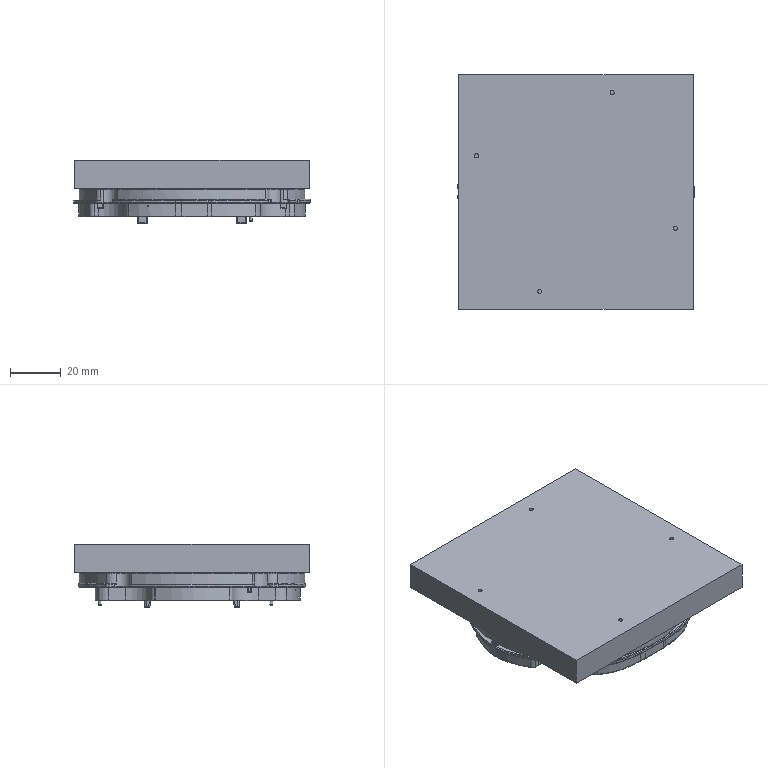NC program | NX | posted with a generic post | part box 92.935 x 92.1 x 24.829 mm
Lines 21645 to 23268 of 39008:
(PLANAR_MILL_7 , TOOL : D4-12-D4-50-3T-FINISH)
N43252 T12 M6
N43254 G54
N43256 G17 G0 G90 X-24.669 Y1.413 S4500 M3
N43258 G43 Z20. H12
N43260 Z-3.025
N43262 G94 G1 Z-6.025 F800.
N43264 X-25.476 Y-0.418
N43266 G2 X-24.68 Y-0.783 R27.9
N43268 G1 Y-0.533
N43270 G2 X-26.282 Y-0.078 R16.4
N43272 X-25.476 Y-0.418 R27.9
N43274 G1 X-26.443 Y-2.614
N43276 G2 X-24.23 Y-3.72 R25.5
N43278 X-22.28 Y-3.348 R12.08
N43280 G1 Y1.507
N43282 G2 X-25.753 Y2.28 R14.
N43284 G1 X-26.121 Y2.413
N43286 G2 X-26.538 Y2.571 R14.
N43288 X-28.778 Y1.718 R25.5
N43290 G3 X-28.876 Y1.255 R9.447
N43292 X-28.981 Y-0.229 R6.65
N43294 X-28.78 Y-1.719 R8.119
N43296 G2 X-26.443 Y-2.614 R25.5
N43298 G1 X-27.41 Y-4.811
N43300 G2 X-24.516 Y-6.338 R23.1
N43302 G1 X-24.286 Y-6.255
N43304 G2 X-20.999 Y-5.68 R9.68
N43306 G1 X-19.88
N43308 Y3.848
N43310 X-20.999
N43312 G2 X-24.938 Y4.537 R11.6
N43314 G1 X-25.306 Y4.67
N43316 G2 X-26.556 Y5.207 R11.6
N43318 X-30.71 Y3.646 R23.1
N43320 G3 X-30.928 Y2.962 R22.542
N43322 X-31.236 Y1.691 R11.847
N43324 X-31.379 Y-0.329 R9.05
N43326 X-31.059 Y-2.504 R10.519
N43328 X-30.726 Y-3.642 R17.948
N43330 G2 X-27.41 Y-4.811 R23.1
N43332 G1 X-28.378 Y-7.007
N43334 G2 X-24.764 Y-9.054 R20.7
N43336 X-23.839 Y-8.646 R7.28
N43338 G1 X-23.471 Y-8.513
N43340 G2 X-20.999 Y-8.08 R7.28
N43342 G1 X-17.999
N43344 G2 X-17.48 Y-8.098 R7.28
N43346 G1 Y6.263
N43348 G2 X-17.999 Y6.248 R9.2
N43350 G1 X-20.999
N43352 G2 X-24.123 Y6.795 R9.2
N43354 G1 X-24.491 Y6.928
N43356 G2 X-26.503 Y7.948 R9.2
N43358 X-32.518 Y5.681 R20.7
N43360 G3 X-33.226 Y3.654 R24.942
N43362 X-33.596 Y2.127 R14.247
N43364 X-33.777 Y-0.429 R11.45
N43366 X-33.383 Y-3.1 R12.919
N43368 X-32.536 Y-5.678 R20.348
N43370 G2 X-28.378 Y-7.007 R20.7
N43372 G1 X-29.345 Y-9.203
N43374 G2 X-24.823 Y-12.047 R18.3
N43376 X-23.024 Y-10.903 R4.88
N43378 G1 X-22.656 Y-10.77
N43380 G2 X-20.999 Y-10.48 R4.88
N43382 G1 X-17.999
N43384 G2 X-16.341 Y-10.77 R4.88
N43386 G1 X-15.973 Y-10.903
N43388 G2 X-15.08 Y-11.332 R4.88
N43390 G1 Y9.277
N43392 G2 X-15.321 Y9.185 R6.8
N43394 G1 X-15.689 Y9.052
N43396 G2 X-17.999 Y8.648 R6.8
N43398 G1 X-20.999
N43400 G2 X-23.308 Y9.052 R6.8
N43402 G1 X-23.676 Y9.185
N43404 G2 X-26.304 Y10.905 R6.8
N43406 X-34.231 Y7.82 R18.3
N43408 G3 X-34.85 Y6.309 R41.541
N43410 X-35.523 Y4.348 R27.342
N43412 X-35.956 Y2.563 R16.647
N43414 X-36.175 Y-0.528 R13.85
N43416 X-35.708 Y-3.696 R15.319
N43418 X-34.584 Y-7.003 R22.748
N43420 X-34.228 Y-7.821 R88.403
N43422 G2 X-29.345 Y-9.203 R18.3
N43424 G1 X-30.313 Y-11.4
N43426 G2 X-23.979 Y-16.442 R15.9
N43428 G1 Y-15.868
N43430 G2 X-23.839 Y-15.047 R2.48
N43432 G1 X-23.707 Y-14.672
N43434 G2 X-22.209 Y-13.16 R2.48
N43436 G1 X-21.841 Y-13.027
N43438 G2 X-20.999 Y-12.88 R2.48
N43440 G1 X-17.999
N43442 G2 X-17.156 Y-13.027 R2.48
N43444 G1 X-16.788 Y-13.16
N43446 G2 X-15.29 Y-14.672 R2.48
N43448 G1 X-15.158 Y-15.047
N43450 G2 X-15.019 Y-15.868 R2.48
N43452 G1 Y-18.001
N43454 G2 X-15.498 Y-19.621 R2.98
N43456 G1 X-7.442 Y-24.843
N43458 G2 X-8.76 Y-26.539 R12.58
N43460 G1 X-8.757 Y-26.548
N43462 G3 X-6.577 Y-26.732 R85.732
N43464 G1 X-5.951 Y-26.774
N43466 X-5.311 Y-26.812
N43468 G3 X-0.977 Y-26.958 R93.406
N43470 X3.366 Y-26.902 R93.502
N43472 X4.427 Y-26.858 R92.619
N43474 X5.477 Y-26.803 R92.484
N43476 X8.597 Y-26.572 R101.654
N43478 G1 X8.778 Y-26.555
N43480 G2 X7.445 Y-24.843 R12.58
N43482 G1 X-7.442
N43484 X-9.456 Y-23.538
N43486 G2 X-11.573 Y-25.897 R10.18
N43488 X-10.67 Y-28.754 R12.7
N43490 G3 X-10.159 Y-28.816 R22.91
N43492 X-6.742 Y-29.126 R88.132
N43494 G1 X-6.102 Y-29.169
N43496 X-5.451 Y-29.208
N43498 G3 X-1.002 Y-29.358 R95.806
N43500 X3.453 Y-29.3 R95.902
N43502 X4.539 Y-29.256 R95.019
N43504 X5.618 Y-29.199 R94.884
N43506 X8.812 Y-28.962 R104.054
N43508 X10.875 Y-28.718 R36.499
N43510 G2 X12.206 Y-26.37 R13.414
N43512 X8.842 Y-22.443 R10.18
N43514 G1 X-8.839
N43516 G2 X-9.456 Y-23.538 R10.18
N43518 G1 X-11.47 Y-22.232
N43520 G2 X-14.799 Y-25.092 R7.78
N43522 X-12.898 Y-30.092 R10.3
N43524 X-12.629 Y-30.858 R11.014
N43526 G3 X-10.423 Y-31.201 R25.31
N43528 X-6.907 Y-31.521 R90.532
N43530 G1 X-6.253 Y-31.564
N43532 X-5.591 Y-31.604
N43534 G3 X-1.028 Y-31.757 R98.206
N43536 X3.539 Y-31.699 R98.302
N43538 X4.652 Y-31.653 R97.419
N43540 X5.758 Y-31.595 R97.284
N43542 X9.026 Y-31.352 R106.454
N43544 X11.881 Y-30.989 R38.899
N43546 X12.634 Y-30.851 R20.991
N43548 G2 X16.026 Y-25.727 R11.014
N43550 G1 X16.029 Y-25.526
N43552 G2 X10.494 Y-20.043 R7.78
N43554 G1 X-10.491
N43556 G2 X-11.47 Y-22.232 R7.78
N43558 G1 X-13.484 Y-20.927
N43560 G2 X-17.999 Y-23.381 R5.38
N43562 G1 X-18.603
N43564 G2 X-18.46 Y-24.767 R18.3
N43566 X-15.26 Y-30.663 R7.9
N43568 X-14.628 Y-32.852 R8.614
N43570 G3 X-13.772 Y-33.068 R18.345
N43572 X-10.686 Y-33.587 R27.71
N43574 X-7.072 Y-33.915 R92.932
N43576 G1 X-6.404 Y-33.959
N43578 X-5.73 Y-34.
N43580 G3 X-1.053 Y-34.157 R100.606
N43582 X3.626 Y-34.097 R100.702
N43584 X4.765 Y-34.05 R99.819
N43586 X5.898 Y-33.991 R99.684
N43588 X9.24 Y-33.743 R108.854
N43590 X12.272 Y-33.357 R41.299
N43592 X14.632 Y-32.842 R23.391
N43594 G2 X18.424 Y-26.925 R8.614
N43596 G1 Y-25.951
N43598 G2 X18.606 Y-23.381 R18.3
N43600 G1 X18.001
N43602 G2 X12.621 Y-18.001 R5.38
N43604 G1 Y-17.643
N43606 X-12.2
N43608 G2 X-12.619 Y-17.613 R2.88
N43610 G1 Y-18.001
N43612 G2 X-13.484 Y-20.927 R5.38
N43614 G1 X-15.498 Y-19.621
N43616 G2 X-17.999 Y-20.981 R2.98
N43618 G1 X-20.999
N43620 G2 X-21.642 Y-20.91 R2.98
N43622 G1 X-21.538 Y-20.442
N43624 G2 X-23.499 Y-18.001 R2.5
N43626 G1 Y-15.868
N43628 G2 X-23.386 Y-15.206 R2.
N43630 G1 X-23.254 Y-14.831
N43632 G2 X-22.046 Y-13.612 R2.
N43634 G1 X-21.678 Y-13.479
N43636 G2 X-20.999 Y-13.36 R2.
N43638 G1 X-17.999
N43640 G2 X-17.319 Y-13.479 R2.
N43642 G1 X-16.951 Y-13.612
N43644 G2 X-15.743 Y-14.831 R2.
N43646 G1 X-15.611 Y-15.206
N43648 G2 X-15.499 Y-15.868 R2.
N43650 G1 Y-18.001
N43652 G2 X-17.999 Y-20.501 R2.5
N43654 G1 X-20.999
N43656 G2 X-21.538 Y-20.442 R2.5
N43658 G1 X-21.642 Y-20.91
N43660 G2 X-20.821 Y-25.951 R15.9
N43662 G1 Y-26.142
N43664 G2 X-17.647 Y-31.234 R5.5
N43666 X-16.952 Y-34.618 R6.214
N43668 G3 X-16.606 Y-34.744 R15.995
N43670 X-14.302 Y-35.409 R20.745
N43672 X-10.95 Y-35.972 R30.11
N43674 X-7.237 Y-36.309 R95.332
N43676 G1 X-6.555 Y-36.355
N43678 X-5.87 Y-36.395
N43680 G3 X-1.078 Y-36.557 R103.006
N43682 X3.712 Y-36.496 R103.102
N43684 X4.877 Y-36.448 R102.219
N43686 X6.039 Y-36.387 R102.084
N43688 X9.455 Y-36.133 R111.254
N43690 X12.663 Y-35.725 R43.699
N43692 X15.887 Y-34.978 R25.791
N43694 X16.955 Y-34.616 R16.039
N43696 G2 X20.824 Y-28.364 R6.214
N43698 G1 Y-25.951
N43700 G2 X21.644 Y-20.91 R15.9
N43702 X21.001 Y-20.981 R2.98
N43704 G1 X18.001
N43706 G2 X15.021 Y-18.001 R2.98
N43708 G1 Y-15.868
N43710 G2 X15.101 Y-15.243 R2.48
N43712 G1 X-12.2
N43714 G2 X-12.68 Y-14.763 R0.48
N43716 G1 Y21.237
N43718 G2 X-12.29 Y21.708 R0.48
N43720 G1 X-13.189 Y26.423
N43722 G2 X-12.2 Y26.517 R5.28
N43724 G1 X15.186
N43726 G2 X14.518 Y27.284 R11.014
N43728 G1 X-14.992
N43730 X-14.954 Y27.209
N43732 G2 X-13.189 Y26.423 R9.7
N43734 G1 X-12.74 Y24.066
N43736 G2 X-12.2 Y24.117 R2.88
N43738 G1 X17.3
N43740 G2 X18.547 Y23.833 R2.88
N43742 X18.424 Y25.95 R18.3
N43744 G1 Y26.923
N43746 G2 X15.936 Y29.418 R8.614
N43748 X15.514 Y29.684 R7.8
N43750 G1 X-18.421
N43752 Y28.077
N43754 G2 X-16.692 Y25.182 R8.8
N43756 X-13.545 Y23.784 R7.3
N43758 X-12.74 Y24.066 R2.88
N43760 G1 X-12.29 Y21.708
N43762 X-12.2 Y21.717
N43764 X17.3
N43766 G2 X17.78 Y21.237 R0.48
N43768 G1 Y20.971
N43770 G2 X18.001 Y20.979 R2.98
N43772 G1 X21.001
N43774 G2 X21.644 Y20.909 R2.98
N43776 G1 X21.541 Y20.441
N43778 G2 X23.501 Y17.999 R2.5
N43780 G1 Y15.956
N43782 G2 X23.389 Y15.294 R2.
N43784 G1 X23.257 Y14.919
N43786 G2 X22.049 Y13.7 R2.
N43788 G1 X21.681 Y13.567
N43790 G2 X21.001 Y13.448 R2.
N43792 G1 X18.001
N43794 G2 X17.3 Y13.575 R2.
N43796 G1 Y-13.487
N43798 X17.322 Y-13.479
N43800 G2 X18.001 Y-13.36 R2.
N43802 G1 X21.001
N43804 G2 X21.681 Y-13.479 R2.
N43806 G1 X22.049 Y-13.612
N43808 G2 X23.257 Y-14.831 R2.
N43810 G1 X23.389 Y-15.206
N43812 G2 X23.501 Y-15.868 R2.
N43814 G1 Y-18.001
N43816 G2 X21.001 Y-20.501 R2.5
N43818 G1 X18.001
N43820 G2 X15.501 Y-18.001 R2.5
N43822 G1 Y-15.868
N43824 G2 X15.614 Y-15.206 R2.
N43826 G1 X15.746 Y-14.831
N43828 X15.771 Y-14.763
N43830 X-12.2
N43832 Y21.237
N43834 X17.3
N43836 Y20.399
N43838 G2 X18.001 Y20.499 R2.5
N43840 G1 X21.001
N43842 G2 X21.541 Y20.441 R2.5
N43844 G1 X21.644 Y20.909
N43846 G2 X20.824 Y25.95 R15.9
N43848 G1 Y28.363
N43850 G2 X17.654 Y31.226 R6.214
N43852 X16.326 Y32.084 R5.4
N43854 G1 X-20.821
N43856 Y27.072
N43858 G2 X-18.61 Y22.899 R6.4
N43860 G1 X-17.999
N43862 G2 X-13.099 Y17.999 R4.9
N43864 G1 Y15.956
N43866 G2 X-13.347 Y14.499 R4.4
N43868 G1 X-13.478 Y14.124
N43870 G2 X-16.136 Y11.443 R4.4
N43872 G1 X-16.504 Y11.31
N43874 G2 X-17.999 Y11.048 R4.4
N43876 G1 X-20.999
N43878 G2 X-22.493 Y11.31 R4.4
N43880 G1 X-22.861 Y11.443
N43882 G2 X-25.519 Y14.124 R4.4
N43884 G1 X-25.66 Y14.528
N43886 G2 X-35.848 Y10.074 R15.9
N43888 G1 X-36.099 Y9.526
N43890 G3 X-37.088 Y7.174 R43.941
N43892 X-37.821 Y5.041 R29.742
N43894 X-38.316 Y2.999 R19.047
N43896 X-38.573 Y-0.628 R16.25
N43898 X-38.033 Y-4.292 R17.719
N43900 X-36.79 Y-7.947 R25.148
N43902 X-35.847 Y-10.075 R90.803
N43904 G2 X-30.313 Y-11.4 R15.9
N43906 G1 X-31.28 Y-13.596
N43908 G2 X-23.221 Y-25.951 R13.5
N43910 G1 Y-28.028
N43912 G2 X-20.121 Y-31.804 R3.1
N43914 X-19.805 Y-35.964 R3.814
N43916 G3 X-17.403 Y-37.008 R18.395
N43918 X-14.833 Y-37.749 R23.145
N43920 X-11.213 Y-38.358 R32.51
N43922 X-7.406 Y-38.703 R97.732
N43924 X-6.706 Y-38.75 R99.978
N43926 X-6.002 Y-38.792 R101.452
N43928 X-1.103 Y-38.957 R105.406
N43930 X3.8 Y-38.894 R105.502
N43932 X4.99 Y-38.845 R104.619
N43934 X6.179 Y-38.782 R104.484
N43936 X9.669 Y-38.524 R113.654
N43938 X13.053 Y-38.093 R46.099
N43940 X16.577 Y-37.277 R28.191
N43942 X19.807 Y-35.963 R18.439
N43944 G2 X23.224 Y-30.314 R3.814
N43946 G1 Y-25.951
N43948 G2 X31.777 Y-13.39 R13.5
N43950 G1 X27.38 Y-2.225
N43952 G2 X28.781 Y-1.72 R25.5
N43954 G3 X28.879 Y-1.256 R9.444
N43956 X28.984 Y0.228 R6.652
N43958 X28.783 Y1.718 R8.116
N43960 G2 X27.38 Y2.224 R25.5
N43962 G1 Y-2.225
N43964 X28.259 Y-4.458
N43966 G2 X30.713 Y-3.647 R23.1
N43968 G3 X30.931 Y-2.963 R22.54
N43970 X31.239 Y-1.692 R11.844
N43972 X31.382 Y0.328 R9.052
N43974 X31.062 Y2.503 R10.516
N43976 X30.729 Y3.641 R17.951
N43978 G2 X24.98 Y6.058 R23.1
N43980 G1 Y-6.059
N43982 G2 X28.259 Y-4.458 R23.1
N43984 G1 X29.139 Y-6.691
N43986 G2 X32.521 Y-5.682 R20.7
N43988 G3 X33.229 Y-3.655 R24.94
N43990 X33.599 Y-2.128 R14.244
N43992 X33.78 Y0.427 R11.452
N43994 X33.386 Y3.099 R12.916
N43996 X32.539 Y5.677 R20.351
N43998 G2 X24.694 Y9.104 R20.7
N44000 X23.842 Y8.734 R7.28
N44002 G1 X23.474 Y8.601
N44004 G2 X22.58 Y8.341 R7.28
N44006 G1 Y-8.253
N44008 G2 X23.474 Y-8.513 R7.28
N44010 G1 X23.842 Y-8.646
N44012 G2 X24.767 Y-9.054 R7.28
N44014 X29.139 Y-6.691 R20.7
N44016 G1 X30.018 Y-8.924
N44018 G2 X34.234 Y-7.821 R18.3
N44020 G3 X34.852 Y-6.31 R41.545
N44022 X35.526 Y-4.349 R27.34
N44024 X35.959 Y-2.564 R16.644
N44026 X36.178 Y0.527 R13.852
N44028 X35.711 Y3.695 R15.316
N44030 X34.587 Y7.001 R22.751
N44032 X34.231 Y7.82 R88.394
N44034 G2 X24.777 Y12.088 R18.3
N44036 X23.027 Y10.991 R4.88
N44038 G1 X22.659 Y10.858
N44040 G2 X21.001 Y10.568 R4.88
N44042 G1 X20.18
N44044 Y-10.48
N44046 X21.001
N44048 G2 X22.659 Y-10.77 R4.88
N44050 G1 X23.027 Y-10.903
N44052 G2 X24.826 Y-12.047 R4.88
N44054 X30.018 Y-8.924 R18.3
N44056 G1 X30.898 Y-11.157
N44058 G2 X35.851 Y-10.075 R15.9
N44060 G1 X36.102 Y-9.527
N44062 G3 X37.091 Y-7.175 R43.945
N44064 X37.824 Y-5.042 R29.74
N44066 X38.319 Y-3. R19.044
N44068 X38.576 Y0.627 R16.252
N44070 X38.036 Y4.291 R17.716
N44072 X36.793 Y7.946 R25.151
N44074 X35.85 Y10.074 R90.794
N44076 G2 X23.981 Y16.44 R15.9
N44078 G1 Y15.956
N44080 G2 X23.842 Y15.135 R2.48
N44082 G1 X23.71 Y14.76
N44084 G2 X22.212 Y13.248 R2.48
N44086 G1 X21.844 Y13.115
N44088 G2 X21.001 Y12.968 R2.48
N44090 G1 X18.001
N44092 G2 X17.78 Y12.978 R2.48
N44094 G1 Y-12.89
N44096 G2 X18.001 Y-12.88 R2.48
N44098 G1 X21.001
N44100 G2 X21.844 Y-13.027 R2.48
N44102 G1 X22.212 Y-13.16
N44104 G2 X23.71 Y-14.672 R2.48
N44106 G1 X23.842 Y-15.047
N44108 G2 X23.981 Y-15.868 R2.48
N44110 G1 Y-16.442
N44112 G2 X30.898 Y-11.157 R15.9
N44114 G1 X31.777 Y-13.39
N44116 G2 X36.724 Y-12.451 R13.5
N44118 G1 X37.385
N44120 G3 X38.287 Y-10.521 R103.509
N44122 X39.329 Y-8.041 R46.345
N44124 X40.122 Y-5.736 R32.14
N44126 X40.679 Y-3.436 R21.444
N44128 X40.974 Y0.726 R18.652
N44130 X40.361 Y4.887 R20.116
N44132 X38.999 Y8.891 R27.551
N44134 X37.386 Y12.45 R93.194
N44136 G1 X36.724
N44138 G2 X23.224 Y25.95 R13.5
N44140 G1 Y30.313
N44142 G2 X19.457 Y33.172 R3.814
N44144 X17.389 Y34.484 R3.
N44146 G1 X-21.326
N44148 G3 X-22.74 Y34.046 R2.5
N44150 X-23.221 Y32.944 R1.5
N44152 G1 Y26.097
N44154 G3 X-22.971 Y25.664 R0.5
N44156 G2 X-21.364 Y20.473 R4.
N44158 X-20.999 Y20.499 R2.5
N44160 G1 X-17.999
N44162 G2 X-15.499 Y17.999 R2.5
N44164 G1 Y15.956
N44166 G2 X-15.611 Y15.294 R2.
N44168 G1 X-15.743 Y14.919
N44170 G2 X-16.951 Y13.7 R2.
N44172 G1 X-17.319 Y13.567
N44174 G2 X-17.999 Y13.448 R2.
N44176 G1 X-20.999
N44178 G2 X-21.678 Y13.567 R2.
N44180 G1 X-22.046 Y13.7
N44182 G2 X-23.254 Y14.919 R2.
N44184 G1 X-23.386 Y15.294
N44186 G2 X-23.499 Y15.956 R2.
N44188 G1 Y17.999
N44190 G2 X-23.448 Y18.501 R2.5
N44192 X-25.349 Y18.218 R4.
N44194 G3 X-25.799 Y18.015 R0.5
N44196 G2 X-36.721 Y12.45 R13.5
N44198 G1 X-37.382
N44200 G3 X-38.284 Y10.52 R103.527
N44202 X-39.327 Y8.04 R46.341
N44204 X-40.119 Y5.735 R32.142
N44206 X-40.676 Y3.435 R21.447
N44208 X-40.971 Y-0.727 R18.65
N44210 X-40.358 Y-4.888 R20.119
N44212 X-38.996 Y-8.892 R27.548
N44214 X-37.383 Y-12.451 R93.203
N44216 G1 X-36.721
N44218 G2 X-31.28 Y-13.596 R13.5
N44220 G1 X-30.474 Y-11.766
N44222 Z-3.025
N44224 G0 Z20.
(PLANAR_MILL_7_COPY_2 , TOOL : D4-12-D4-50-3T-FINISH)
N44226 X0.103 Y-27.363
N44228 Z-3.525
N44230 G1 Z-6.525
N44232 X0.105 Y-29.363
N44234 G3 X3.453 Y-29.3 R95.902
N44236 X4.539 Y-29.256 R95.019
N44238 X5.618 Y-29.199 R94.884
N44240 X7.299 Y-29.088 R116.954
N44242 X8.868 Y-28.954 R65.735
N44244 X10.877 Y-28.711 R43.493
N44246 G2 X11.209 Y-28.014 R13.414
N44248 X9.478 Y-26.589 R12.1
N44250 G1 X-9.475
N44252 G2 X-10.892 Y-27.793 R12.1
N44254 X-10.67 Y-28.752 R12.7
N44256 G3 X-10.023 Y-28.831 R24.468
N44258 X-6.743 Y-29.126 R89.057
N44260 G1 X-6.102 Y-29.169
N44262 X-5.447 Y-29.208
N44264 G3 X-1.002 Y-29.358 R95.806
N44266 X0.105 Y-29.363 R95.902
N44268 G1 X0.108 Y-31.763
N44270 G3 X3.539 Y-31.699 R98.302
N44272 X4.652 Y-31.653 R97.419
N44274 X5.758 Y-31.595 R97.284
N44276 X7.474 Y-31.482 R119.354
N44278 X9.101 Y-31.343 R68.135
N44280 X12.393 Y-30.902 R45.893
N44282 G1 X12.632 Y-30.859
N44284 G2 X14.662 Y-27.108 R11.014
N44286 X10.532 Y-24.189 R9.7
N44288 G1 X-10.529
N44290 G2 X-13.82 Y-26.755 R9.7
N44292 X-12.898 Y-30.092 R10.3
N44294 X-12.629 Y-30.857 R11.014
N44296 G3 X-10.282 Y-31.217 R26.868
N44298 X-6.908 Y-31.521 R91.457
N44300 G1 X-6.253 Y-31.564
N44302 X-5.586 Y-31.604
N44304 G3 X-1.028 Y-31.757 R98.206
N44306 X0.108 Y-31.763 R98.302
N44308 G1 X0.111 Y-34.163
N44310 G3 X3.626 Y-34.097 R100.702
N44312 X4.765 Y-34.05 R99.819
N44314 X5.898 Y-33.991 R99.684
N44316 X7.649 Y-33.875 R121.754
N44318 X9.333 Y-33.732 R70.535
N44320 X12.797 Y-33.267 R48.293
N44322 X14.63 Y-32.855 R18.15
N44324 G2 X18.424 Y-26.925 R8.614
N44326 G1 Y-25.951
N44328 G2 X18.436 Y-25.301 R18.3
N44330 G1 X18.001
N44332 G2 X11.762 Y-21.789 R7.3
N44334 G1 X-11.759
N44336 G2 X-17.813 Y-25.298 R7.3
N44338 X-15.26 Y-30.663 R7.9
N44340 X-14.627 Y-32.854 R8.614
N44342 G3 X-13.536 Y-33.12 R20.526
N44344 X-10.541 Y-33.603 R29.268
N44346 X-7.073 Y-33.915 R93.857
N44348 G1 X-6.404 Y-33.959
N44350 X-5.726 Y-34.
N44352 G3 X-1.053 Y-34.157 R100.606
N44354 X0.111 Y-34.163 R100.702
N44356 G1 X0.114 Y-36.563
N44358 G3 X3.712 Y-36.496 R103.102
N44360 X4.877 Y-36.448 R102.219
N44362 X6.039 Y-36.387 R102.084
N44364 X7.824 Y-36.269 R124.154
N44366 X9.566 Y-36.12 R72.935
N44368 X13.202 Y-35.633 R50.693
N44370 X16.376 Y-34.825 R20.55
N44372 X16.955 Y-34.616 R17.313
N44374 G2 X20.824 Y-28.364 R6.214
N44376 G1 Y-25.951
N44378 G2 X21.12 Y-22.899 R15.9
N44380 G1 X18.001 Y-22.901
N44382 G2 X13.302 Y-19.389 R4.9
N44384 G1 X-13.299
N44386 G2 X-17.999 Y-22.901 R4.9
N44388 G1 X-21.117 Y-22.899
N44390 G2 X-20.821 Y-25.951 R15.9
N44392 G1 Y-26.142
N44394 G2 X-17.647 Y-31.234 R5.5
N44396 X-16.952 Y-34.618 R6.214
N44398 G3 X-16.378 Y-34.826 R17.312
N44400 X-15.24 Y-35.175 R18.745
N44402 X-14.041 Y-35.466 R22.926
N44404 X-10.8 Y-35.989 R31.668
N44406 X-7.238 Y-36.309 R96.257
N44408 G1 X-6.555 Y-36.355
N44410 X-5.865 Y-36.396
N44412 G3 X-1.078 Y-36.557 R103.006
N44414 X0.114 Y-36.563 R103.102
N44416 G1 X0.116 Y-38.963
N44418 G3 X3.8 Y-38.894 R105.502
N44420 X4.99 Y-38.845 R104.619
N44422 X6.179 Y-38.782 R104.484
N44424 X7.999 Y-38.662 R126.554
N44426 X9.798 Y-38.509 R75.335
N44428 X13.606 Y-37.999 R53.093
N44430 X17.152 Y-37.097 R22.95
N44432 X18.506 Y-36.578 R19.713
N44434 X19.807 Y-35.962 R18.287
N44436 G1 X19.795 Y-35.941
N44438 G2 X23.224 Y-30.314 R3.814
N44440 G1 Y-25.951
N44442 G2 X26.628 Y-16.989 R13.5
N44444 G1 X23.501
N44446 Y-18.001
N44448 G2 X21.001 Y-20.501 R2.5
N44450 G1 X18.001
N44452 G2 X15.501 Y-18.001 R2.5
N44454 G1 Y-16.989
N44456 X-15.499
N44458 Y-18.001
N44460 G2 X-17.999 Y-20.501 R2.5
N44462 G1 X-20.999
N44464 G2 X-23.499 Y-18.001 R2.5
N44466 G1 Y-16.989
N44468 X-26.625
N44470 G2 X-23.221 Y-25.951 R13.5
N44472 G1 Y-28.028
N44474 G2 X-20.121 Y-31.804 R3.1
N44476 X-19.805 Y-35.964 R3.814
N44478 G3 X-18.506 Y-36.579 R18.312
N44480 X-17.154 Y-37.097 R19.712
N44482 X-15.87 Y-37.49 R21.145
N44484 X-14.545 Y-37.813 R25.326
N44486 X-11.059 Y-38.375 R34.068
N44488 X-7.407 Y-38.703 R98.657
N44490 X-6.706 Y-38.75 R101.242
N44492 X-6.002 Y-38.792 R105.477
N44494 X-1.103 Y-38.957 R105.406
N44496 X0.116 Y-38.963 R105.502
N44498 G1 X0.114 Y-36.963
N44500 Z-3.525
N44502 G0 Z20.
(PLANAR_MILL_7_COPY , TOOL : D4-12-D4-50-3T-FINISH)
N44504 X1.8 Y7.097
N44506 Z-5.125
N44508 G1 Y-0.763 Z-5.813
N44510 X3.3 Z-5.944
N44512 Y7.237 Z-6.644
N44514 X1.8 Z-6.776
N44516 Y3.237 Z-7.125
N44518 Y-0.763
N44520 X3.3
N44522 Y7.237
N44524 X1.8
N44526 Y3.237
N44528 X-0.6
N44530 Y-3.163
N44532 X5.7
N44534 Y9.637
N44536 X-0.6
N44538 Y3.237
N44540 X-3.
N44542 Y-5.563
N44544 X8.1
N44546 Y12.037
N44548 X-3.
N44550 Y3.237
N44552 X-5.4
N44554 Y-7.963
N44556 X10.5
N44558 Y14.437
N44560 X-5.4
N44562 Y3.237
N44564 X-7.8
N44566 Y-10.363
N44568 X12.9
N44570 Y16.837
N44572 X-7.8
N44574 Y3.237
N44576 X-10.2
N44578 Y-12.763
N44580 X15.3
N44582 Y19.237
N44584 X-10.2
N44586 Y3.237
N44588 Z-5.125
N44590 G0 Z20.
(PLANAR_MILL_8 , TOOL : D4-12-D4-50-3T-FINISH)
N44592 X2.722 Y-46.43
N44594 Z-5.025
N44596 G1 Z-8.025
N44598 X2.674 Y-44.431
N44600 G2 X-1.16 Y-44.457 R110.96
N44602 X-6.314 Y-44.283 R110.965
N44604 X-7.052 Y-44.239 R108.655
N44606 X-7.793 Y-44.19 R106.796
N44608 X-12.102 Y-43.79 R97.842
N44610 X-16.511 Y-43.005 R36.323
N44612 X-21.497 Y-41.252 R26.415
N44614 X-26.037 Y-38.46 R23.641
N44616 X-28.721 Y-32.949 R7.
N44618 G1 Y-25.951
N44620 G3 X-36.721 Y-17.951 R8.
N44622 G1 X-38.324
N44624 G2 X-41.921 Y-15.701 R4.
N44626 G1 X-42.093 Y-15.347
N44628 G2 X-43.314 Y-12.745 R107.036
N44630 X-44.45 Y-10.043 R52.936
N44632 X-45.371 Y-7.379 R38.019
N44634 X-46.063 Y-4.58 R26.791
N44636 X-46.464 Y1.056 R24.133
N44638 X-45.59 Y6.612 R25.715
N44640 X-43.934 Y11.334 R34.882
N44642 X-41.911 Y15.713 R101.663
N44644 X-38.321 Y17.95 R4.
N44646 G1 X-36.721
N44648 G3 X-28.721 Y25.95 R8.
N44650 G1 Y32.944
N44652 G2 X-26.183 Y38.338 R7.
N44654 G1 X-26.103 Y38.401
N44656 G2 X-21.637 Y39.978 R8.
N44658 G1 X-21.559 Y39.98
N44660 X21.332 Y39.984
N44662 G2 X26.107 Y38.403 R8.
N44664 G1 X26.189 Y38.339
N44666 G2 X28.724 Y32.947 R7.
N44668 G1 Y25.95
N44670 G3 X36.724 Y17.95 R8.
N44672 G1 X38.327
N44674 G2 X41.924 Y15.7 R4.
N44676 G1 X42.095 Y15.346
N44678 G2 X43.551 Y12.221 R104.577
N44680 X44.864 Y8.936 R45.111
N44682 X45.986 Y4.954 R31.184
N44684 X46.492 Y0.735 R23.963
N44686 G1 X46.504 Y0.002
N44688 X46.491 Y-0.763
N44690 G2 X46.117 Y-4.284 R23.947
N44692 X45.283 Y-7.675 R28.662
N44694 X43.727 Y-11.824 R38.944
N44696 X41.914 Y-15.714 R105.253
N44698 X38.324 Y-17.951 R4.
N44700 G1 X36.724
N44702 G3 X28.724 Y-25.951 R8.
N44704 G1 Y-32.946
N44706 G2 X26.04 Y-38.457 R7.
N44708 X23.669 Y-40.095 R24.159
N44710 X21.116 Y-41.439 R23.832
N44712 X18.415 Y-42.471 R24.557
N44714 X15.659 Y-43.199 R29.764
N44716 X11.031 Y-43.918 R41.738
N44718 X6.5 Y-44.273 R115.493
N44720 G1 X6.313 Y-44.284
N44722 X6.125 Y-44.294
N44724 X6. Y-44.301
N44726 X5.875 Y-44.308
N44728 X5.749 Y-44.314
N44730 G2 X5.499 Y-44.327 R110.292
N44732 G1 X5.374 Y-44.333
N44734 G2 X5.123 Y-44.345 R110.244
N44736 X4.372 Y-44.377 R110.125
N44738 X4.122 Y-44.386 R110.403
N44740 X2.674 Y-44.431 R110.96
N44742 G1 X2.722 Y-46.43
N44744 Z-5.025
N44746 G0 Z20.
(PLANAR_MILL_8_COPY , TOOL : D4-12-D4-50-3T-FINISH)
N44748 X-35.918 Y-27.373
N44750 Z-5.025
N44752 G1 Z-8.025
N44754 Y-25.373
N44756 X-36.918
N44758 G2 X-39.193 Y-23.098 R2.275
N44760 G1 Y-22.098
N44762 G2 X-36.918 Y-19.823 R2.275
N44764 G1 X-34.918
N44766 G2 X-32.643 Y-22.098 R2.275
N44768 G1 Y-23.098
N44770 G2 X-34.918 Y-25.373 R2.275
N44772 G1 X-35.918
N44774 Y-27.373
N44776 Z-5.025
N44778 G0 Z20.
N44780 X35.921
N44782 Z-5.025
N44784 G1 Z-8.025
N44786 Y-25.373
N44788 X34.921
N44790 G2 X32.646 Y-23.098 R2.275
N44792 G1 Y-22.098
N44794 G2 X34.921 Y-19.823 R2.275
N44796 G1 X36.921
N44798 G2 X39.196 Y-22.098 R2.275
N44800 G1 Y-23.098
N44802 G2 X36.921 Y-25.373 R2.275
N44804 G1 X35.921
N44806 Y-27.373
N44808 Z-5.025
N44810 G0 Z20.
(FLOOR_FACING_1 , TOOL : D4-12-D4-50-3T-FINISH)
N44812 X-44.494 Y-20.992
N44814 Z-5.025
N44816 G1 Z-8.025
N44818 X-40.117 Y-18.592
N44820 G2 X-38.76 Y-18.988 R1.
N44822 G1 X-38.115 Y-20.164
N44824 G2 X-36.918 Y-19.823 R2.275
N44826 G1 X-34.918
N44828 G2 X-32.643 Y-22.098 R2.275
N44830 G1 Y-22.907
N44832 G2 X-28.724 Y-25.755 R5.1
N44834 G3 X-36.721 Y-17.951 R8.
N44836 G1 X-38.324
N44838 G2 X-39.392 Y-17.806 R4.
N44840 G1 X-38.901 Y-18.731
N44842 X-38.76 Y-18.988
N44844 X-38.279 Y-19.865
N44846 G2 X-37.9 Y-19.812 R0.5
N44848 G1 X-43.475 Y-22.869
N44850 Z-5.025
N44852 G0 Z20.
N44854 X-12.095 Y48.505
N44856 Z-5.025
N44858 G1 Z-8.025
N44860 X-11.515 Y43.539
N44862 G2 X-12.392 Y42.43 R1.
N44864 G3 X-21.139 Y39.98 R27.062
N44866 G1 X21.106 Y39.984
N44868 X19.973 Y40.518
N44870 X18.048 Y41.221
N44872 X16.06 Y41.768
N44874 X14.018 Y42.185
N44876 X11.935 Y42.495
N44878 X9.825 Y42.722
N44880 X7.7 Y42.892
N44882 X3.303 Y43.107
N44884 Y41.583
N44886 X-3.297
N44888 Y43.111
N44890 X-6.417 Y42.974
N44892 X-9.758 Y42.737
N44894 X-12.392 Y42.43
N44896 X-13.067 Y42.351
N44898 X-13.383 Y42.295
N44900 G2 X-14.544 Y43.102 R1.
N44902 G1 X-15.427 Y48.023
N44904 Z-5.025
N44906 G0 Z20.
N44908 X34.277 Y36.865
N44910 Z-5.025
N44912 G1 Z-8.025
N44914 X30.54 Y33.549
N44916 G2 X29.129 Y33.633 R1.
N44918 G1 X28.608 Y34.22
N44920 G2 X28.724 Y32.947 R7.
N44922 G1 Y30.163
N44924 G2 X29.606 Y31.452 R5.1
N44926 G3 X29.65 Y33.046 R1.2
N44928 G1 X29.129 Y33.633
N44930 X28.608 Y34.22
N44932 G2 X28.644 Y34.008 R7.
N44934 G1 Z-5.025
N44936 G0 Z20.
N44938 X42.761 Y24.144
N44940 Z-5.025
N44942 G1 Z-8.025
N44944 X35.869 Y20.188
N44946 G3 X35.82 Y20.568 R0.5
N44948 G1 X35.581 Y20.983
N44950 X35.359 Y21.367
N44952 G2 X32.894 Y21.074 R6.9
N44954 G3 X36.276 Y19.766 R6.2
N44956 G1 X36.046 Y20.174
N44958 X35.82 Y20.568
N44960 X37.381 Y21.464
N44962 X37.14 Y21.883
N44964 X36.667 Y22.7
N44966 G3 X35.19 Y23.214 R1.2
N44968 G2 X28.727 Y25.753 R5.1
N44970 G3 X36.724 Y17.95 R8.
N44972 G1 X38.327
N44974 G2 X39.395 Y17.804 R4.
N44976 G1 X37.381 Y21.464
N44978 X37.14 Y21.883
N44980 X36.881 Y22.33
N44982 G2 X37.245 Y23.697 R1.
N44984 G1 X41.55 Y26.193
N44986 Z-5.025
N44988 G0 Z20.
N44990 X43.559 Y-22.72
N44992 Z-5.025
N44994 G1 Z-8.025
N44996 X39.165 Y-20.343
N44998 G2 X38.761 Y-18.988 R1.
N45000 G1 X39.392 Y-17.806
N45002 G2 X38.324 Y-17.951 R4.
N45004 G1 X36.724
N45006 G3 X28.727 Y-25.755 R8.
N45008 G2 X32.646 Y-22.907 R5.1
N45010 G1 Y-22.098
N45012 G2 X34.921 Y-19.823 R2.275
N45014 G1 X36.921
N45016 G2 X38.116 Y-20.162 R2.275
N45018 G1 X38.761 Y-18.988
N45020 X38.92 Y-18.693
N45022 X39.233 Y-18.106
N45024 G2 X39.909 Y-17.898 R0.5
N45026 G1 X44.769 Y-20.467
N45028 Z-5.025
N45030 G0 Z20.
N45032 X32.999 Y-38.314
N45034 Z-5.025
N45036 G1 Z-8.025
N45038 X29.231 Y-35.032
N45040 G2 X29.134 Y-33.621 R1.
N45042 G1 X29.661 Y-33.016
N45044 G3 X29.6 Y-31.446 R1.2
N45046 G2 X28.724 Y-30.164 R5.1
N45048 G1 Y-32.946
N45050 G2 X28.606 Y-34.227 R7.
N45052 G1 X29.134 Y-33.621
N45054 X29.661 Y-33.016
N45056 X29.771 Y-32.853
N45058 G2 X31.132 Y-32.469 R1.
N45060 G1 X35.433 Y-34.879
N45062 Z-5.025
N45064 G0 Z20.
N45066 X-34.224 Y-36.914
N45068 Z-5.025
N45070 G1 Z-8.025
N45072 X-30.553 Y-33.573
N45074 G2 X-29.14 Y-33.64 R1.
N45076 G1 X-28.603 Y-34.232
N45078 G2 X-28.721 Y-32.949 R7.
N45080 G1 Y-30.164
N45082 G2 X-29.599 Y-31.448 R5.1
N45084 G3 X-29.653 Y-33.026 R1.2
N45086 G1 X-29.387 Y-33.348
N45088 X-29.14 Y-33.64
N45090 X-28.603 Y-34.232
N45092 G2 X-28.637 Y-34.034 R7.
N45094 G1 Z-5.025
N45096 G0 Z20.
N45098 X-42.391 Y24.778
N45100 Z-5.025
N45102 G1 Z-8.025
N45104 X-35.512 Y20.802
N45106 G3 X-35.814 Y20.568 R0.5
N45108 G1 X-36.116 Y20.041
N45110 X-36.271 Y19.766
N45112 G3 X-32.892 Y21.074 R6.2
N45114 G2 X-35.353 Y21.366 R6.9
N45116 G1 X-35.446 Y21.207
N45118 X-35.814 Y20.568
N45120 X-37.377 Y21.462
N45122 X-39.388 Y17.805
N45124 G2 X-38.321 Y17.95 R4.
N45126 G1 X-36.721
N45128 G3 X-28.724 Y25.753 R8.
N45130 G2 X-35.184 Y23.213 R5.1
N45132 G3 X-36.659 Y22.7 R1.2
N45134 G1 X-37.003 Y22.109
N45136 X-37.377 Y21.462
N45138 X-37.681 Y20.93
N45140 X-37.871 Y20.593
N45142 G2 X-39.234 Y20.213 R1.
N45144 G1 X-43.584 Y22.669
N45146 Z-5.025
N45148 G0 Z20.
N45150 X-33.03 Y38.296
N45152 Z-5.025
N45154 G1 Z-8.025
N45156 X-29.236 Y35.044
N45158 G2 X-29.127 Y33.634 R1.
N45160 G1 X-29.656 Y33.017
N45162 G3 X-29.597 Y31.445 R1.2
N45164 G2 X-28.721 Y30.163 R5.1
N45166 G1 Y32.944
N45168 G2 X-28.598 Y34.251 R7.
N45170 G1 X-29.127 Y33.634
N45172 X-29.656 Y33.017
N45174 X-29.762 Y32.863
N45176 G2 X-31.127 Y32.494 R1.
N45178 G1 X-35.402 Y34.949
N45180 Z-5.025
N45182 G0 Z20.
(PLANAR_MILL_10 , TOOL : D4-12-D4-50-3T-FINISH)
N45184 X-18.729 Y32.784
N45186 Z0.375
N45188 G1 Z-2.625
N45190 Y36.784
N45192 X-20.729
N45194 X-21.326
N45196 G3 X-24.167 Y35.853 R4.8
N45198 X-25.521 Y32.944 R3.8
N45200 G1 Y26.097
N45202 G3 X-24.121 Y23.672 R2.8
N45204 G2 X-25.132 Y20.507 R1.7
N45206 G3 X-27.659 Y19.369 R2.8
N45208 G2 X-36.721 Y14.75 R11.2
N45210 G1 X-38.009
N45212 G3 X-39.177 Y14.019 R1.3
N45214 X-41.384 Y9.107 R85.691
N45216 X-42.913 Y3.969 R26.452
N45218 X-43.284 Y-0.191 R21.168
N45220 X-42.84 Y-4.345 R21.641
N45222 X-41.331 Y-9.25 R26.958
N45224 X-39.18 Y-14.02 R88.056
N45226 X-38.011 Y-14.751 R1.3
N45228 G1 X-36.721
N45230 G2 X-25.521 Y-25.951 R11.2
N45232 G1 Y-28.591
N45234 G3 X-25.231 Y-29.572 R1.8
N45236 G1 Z0.375
N45238 G0 Z20.
N45240 X-18.354 Y-31.4
N45242 Z0.375
N45244 G1 Z-2.625
N45246 X-21.835 Y-33.371
N45248 G2 X-21.82 Y-34.856 R1.514
N45250 G3 X-20.869 Y-38.003 R2.3
N45252 X-18.998 Y-38.862 R20.233
N45254 X-17.054 Y-39.54 R23.615
N45256 X-12.359 Y-40.53 R28.493
N45258 X-6.133 Y-41.088 R91.573
N45260 X-3.295 Y-41.212 R107.536
N45262 X-2.908 Y-41.224 R107.659
N45264 X1.456 Y-41.253 R107.441
N45266 X3.882 Y-41.193 R107.66
N45268 X4.464 Y-41.17 R107.763
N45270 X6.313 Y-41.078 R105.797
N45272 X8.558 Y-40.928 R137.244
N45274 X10.798 Y-40.722 R67.482
N45276 X15.976 Y-39.829 R42.061
N45278 X20.871 Y-38.001 R21.135
N45280 X21.823 Y-34.855 R2.3
N45282 G2 X23.179 Y-32.613 R1.514
N45284 G3 X25.524 Y-30.314 R2.3
N45286 G1 Y-25.951
N45288 G2 X36.724 Y-14.751 R11.2
N45290 G1 X38.012
N45292 G3 X39.18 Y-14.021 R1.3
N45294 X41.414 Y-9.038 R84.756
N45296 X42.943 Y-3.824 R26.205
N45298 X43.287 Y0.263 R21.075
N45300 X42.843 Y4.343 R21.659
N45302 X41.334 Y9.248 R26.963
N45304 X39.183 Y14.018 R88.065
N45306 X38.014 Y14.75 R1.3
N45308 G1 X36.724
N45310 G2 X25.524 Y25.95 R11.2
N45312 G1 Y30.313
N45314 G3 X23.179 Y32.612 R2.3
N45316 G2 X21.652 Y33.904 R1.514
N45318 G1 X21.637 Y33.993
N45320 X18.164 Y31.769
N45322 Z0.375
N45324 G0 Z20.
N45326 X16.601 Y32.784
N45328 Z0.375
N45330 G1 Z-2.625
N45332 X17.634 Y36.784
N45334 X-13.201
N45336 X-15.201
N45338 Y32.784
N45340 Z0.375
N45342 G0 Z20.
(FLOOR_FACING_1_COPY , TOOL : D4-12-D4-50-3T-FINISH)
N45344 X-27.79 Y-40.516
N45346 Z0.375
N45348 G1 Z-2.625
N45350 X-24.933 Y-36.43
N45352 G2 X-23.54 Y-36.184 R1.
N45354 G1 X-23.057 Y-36.521
N45356 G2 X-22.696 Y-34.374 R3.3
N45358 G3 X-22.752 Y-33.798 R0.514
N45360 G1 X-22.828 Y-33.707
N45362 G2 X-25.421 Y-32.385 R2.6
N45364 G1 Y-32.949
N45366 G3 X-24.022 Y-35.846 R3.7
N45368 G1 X-23.54 Y-36.184
N45370 X-23.057 Y-36.521
N45372 G2 X-23.101 Y-36.112 R3.3
N45374 X-22.147 Y-35.069 R1.
N45376 G1 X-16.67 Y-34.822
N45378 Z0.375
N45380 G0 Z20.
N45382 X30.251 Y29.208
N45384 Z0.375
N45386 G1 Z-2.625
N45388 X22.962 Y33.13
N45390 G2 X22.555 Y34.485 R1.
N45392 G1 X22.645 Y34.026
N45394 G3 X23.159 Y33.612 R0.514
N45396 G2 X25.424 Y32.772 R3.3
N45398 G1 Y32.947
N45400 G3 X24.11 Y35.776 R3.7
N45402 X22.726 Y36.473 R4.7
N45404 G2 X22.465 Y34.943 R2.6
N45406 G1 X22.555 Y34.485
N45408 X22.645 Y34.026
N45410 G3 X22.978 Y33.641 R0.514
N45412 G2 X23.588 Y32.365 R1.
N45414 G1 X21.95 Y27.723
N45416 Z0.375
N45418 G0 Z20.
N45420 X-31.426 Y25.309
N45422 Z0.375
N45424 G1 Z-2.625
N45426 X-26.605 Y23.771
N45428 G2 X-25.956 Y22.514 R1.
N45430 X-26.383 Y21.389 R11.3
N45432 X-25.038 Y21.503 R3.8
N45434 G3 X-24.621 Y22.806 R0.7
N45436 G2 X-25.652 Y23.678 R3.8
N45438 X-25.956 Y22.514 R11.3
N45440 X-26.302 Y21.576 R11.3
N45442 X-27.611 Y21.041 R1.
N45444 G1 X-32.174 Y22.957
N45446 Z0.375
N45448 G0 Z20.
N45450 X26.133 Y-41.666
N45452 Z0.375
N45454 G1 Z-2.625
N45456 X23.292 Y-37.568
N45458 G2 X23.544 Y-36.177 R1.
N45460 G1 X24.027 Y-35.842
N45462 G3 X25.424 Y-32.946 R3.7
N45464 G1 Y-32.773
N45466 G2 X23.159 Y-33.613 R3.3
N45468 G3 X22.699 Y-34.374 R0.514
N45470 G2 X23.061 Y-36.512 R3.3
N45472 G1 X23.544 Y-36.177
N45474 X24.027 Y-35.842
N45476 G3 X24.335 Y-35.568 R3.7
N45478 G2 X25.749 Y-35.571 R1.
N45480 G1 X29.24 Y-39.078
N45482 Z0.375
N45484 G0 Z20.
(FLOOR_FACING_1_COPY_COPY , TOOL : D4-12-D4-50-3T-FINISH)
N45486 X31.946 Y-22.073
N45488 Z-4.025
N45490 G1 Z-6.025
N45492 G3 X32.946 Y-23.073 R1.
N45494 G1 X38.896
N45496 G3 X39.896 Y-22.073 R1.
N45498 G1 Z-4.025
N45500 G0 Z20.
N45502 X14.801 Y-16.866
N45504 Z2.
N45506 G1 Z0.
N45508 G3 X15.801 Y-17.866 R1.
N45510 G1 X23.201
N45512 G3 X24.201 Y-16.866 R1.
N45514 G1 Z2.
N45516 G0 Z20.
N45518 X14.801 Y18.199
N45520 Z2.
N45522 G1 Z0.
N45524 G3 X15.801 Y17.199 R1.
N45526 G1 X23.201
N45528 G3 X24.201 Y18.199 R1.
N45530 G1 Z2.
N45532 G0 Z20.
N45534 X16.7 Y36.718
N45536 Z0.975
N45538 G1 Z-1.025
N45540 Y36.625
N45542 G3 X17.7 Y35.625 R1.
N45544 G1 X22.599 Y35.626
N45546 G3 X23.599 Y36.626 R1.
N45548 G1 Y36.718
N45550 Z0.975
N45552 G0 Z20.
N45554 X-24.199 Y18.199
N45556 Z2.
N45558 G1 Z0.
N45560 G3 X-23.199 Y17.199 R1.
N45562 G1 X-15.799
N45564 G3 X-14.799 Y18.199 R1.
N45566 G1 Z2.
N45568 G0 Z20.
N45570 X-24.199 Y-16.866
N45572 Z2.
N45574 G1 Z0.
N45576 G3 X-23.199 Y-17.866 R1.
N45578 G1 X-15.799
N45580 G3 X-14.799 Y-16.866 R1.
N45582 G1 Z2.
N45584 G0 Z20.
N45586 X-26.596 Y-30.534
N45588 Z0.975
N45590 G1 Z-1.025
N45592 Y-30.627
N45594 G3 X-25.596 Y-31.627 R1.
N45596 G1 X-20.697
N45598 G3 X-19.697 Y-30.626 R1.
N45600 G1 Y-30.534
N45602 Z0.975
N45604 G0 Z20.
N45606 X-39.893 Y-22.073
N45608 Z-4.025
N45610 G1 Z-6.025
N45612 G3 X-38.893 Y-23.073 R1.
N45614 G1 X-32.943
N45616 G3 X-31.943 Y-22.073 R1.
N45618 G1 Z-4.025
N45620 G0 Z20.
(PLANAR_MILL_10_COPY , TOOL : D4-12-D4-50-3T-FINISH)
N45622 X15.549 Y34.125
N45624 Z-0.625
N45626 G1 Z-2.625
N45628 G3 X17.549 Y36.125 R2.
N45630 G2 X20.149 Y38.725 R2.6
N45632 X17.549 Y36.125 R-2.6
N45634 G3 X15.549 Y38.125 R2.
N45636 G1 Z-0.625
N45638 G0 Z20.
N45640 X-18.546 Y-29.127
N45642 Z-0.625
N45644 G1 Z-2.625
N45646 G3 X-20.546 Y-31.127 R2.
N45648 G2 X-23.146 Y-33.727 R2.6
N45650 X-20.546 Y-31.127 R-2.6
N45652 G3 X-18.546 Y-33.127 R2.
N45654 G1 Z-0.625
N45656 G0 Z20.
(PLANAR_MILL_11 , TOOL : D4-12-D4-50-3T-FINISH)
N45658 X-22.675 Y40.939
N45660 Z-2.125
N45662 G1 Z-4.125
N45664 G3 X-21.637 Y39.978 R1.
N45666 G2 X-18.612 Y37.719 R3.
N45668 G1 X-18.564 Y37.562
N45670 G2 X-18.429 Y36.784 R2.3
N45672 G1 X-15.501
N45674 G2 X-15.366 Y37.562 R2.3
N45676 G1 X-15.317 Y37.72
N45678 G2 X-12.409 Y39.984 R3.
N45680 G3 X-11.409 Y40.984 R1.
N45682 G1 Z-2.125
N45684 G0 Z20.
(PLANAR_MILL_11_COPY , TOOL : D4-12-D4-50-3T-FINISH)
N45686 X-22.675 Y40.939
N45688 Z-2.125
N45690 G1 Z-4.125
N45692 G3 X-21.637 Y39.978 R1.
N45694 G2 X-18.612 Y37.719 R3.
N45696 G1 X-18.564 Y37.562
N45698 G2 X-20.729 Y34.484 R2.3
N45700 G3 X-21.729 Y33.484 R1.
N45702 G1 Z-2.125
N45704 G0 Z20.
N45706 X-12.201
N45708 Z-2.125
N45710 G1 Z-4.125
N45712 G3 X-13.201 Y34.484 R1.
N45714 G2 X-15.366 Y37.562 R2.3
N45716 G1 X-15.317 Y37.72
N45718 G2 X-12.409 Y39.984 R3.
N45720 G3 X-11.409 Y40.984 R1.
N45722 G1 Z-2.125
N45724 G0 Z20.
N45726 M5
(PLANAR_MILL_7_COPY_1 , TOOL : D3-9-D4-50-3T-ROUGH)
N45728 T15 M6
N45730 G54
N45732 G17 G0 G90 X0.001 Y-37.963 S4500 M3
N45734 G43 Z20. H15
N45736 Z-3.025
N45738 G94 G1 Z-6.025 F600.
N45740 Y-39.463
N45742 G3 X3.818 Y-39.394 R106.002
N45744 X5.013 Y-39.345 R105.119
N45746 X6.208 Y-39.282 R104.984
N45748 X9.714 Y-39.022 R114.154
N45750 X13.134 Y-38.587 R46.599
N45752 X16.721 Y-37.756 R28.691
N45754 X20.038 Y-36.406 R18.939
N45756 X20.245 Y-35.722 R0.5
N45758 G2 X23.215 Y-30.814 R3.314
N45760 G3 X23.724 Y-30.314 R0.5
N45762 G1 Y-25.951
N45764 G2 X36.724 Y-12.951 R13.
N45766 G1 X37.699
N45768 G3 X38.742 Y-10.728 R104.009
N45770 X39.796 Y-8.221 R46.845
N45772 X40.6 Y-5.88 R32.64
N45774 X41.171 Y-3.527 R21.944
N45776 X41.473 Y0.747 R19.152
N45778 X40.845 Y5.011 R20.616
N45780 X39.459 Y9.088 R28.051
N45782 X37.701 Y12.95 R93.694
N45784 G1 X36.724
N45786 G2 X23.724 Y25.95 R13.
N45788 G1 Y30.313
N45790 G3 X23.215 Y30.813 R0.5
N45792 G2 X19.871 Y33.641 R3.314
N45794 X17.674 Y34.984 R2.5
N45796 G1 X-21.326
N45798 G3 X-23.051 Y34.438 R3.
N45800 X-23.721 Y32.944 R2.
N45802 G1 Y26.097
N45804 G3 X-23.221 Y25.231 R1.
N45806 G2 X-25.302 Y18.715 R3.5
N45808 G3 X-26.203 Y18.31 R1.
N45810 G2 X-36.721 Y12.95 R13.
N45812 G1 X-37.696
N45814 G3 X-38.739 Y10.727 R104.027
N45816 X-39.793 Y8.22 R46.841
N45818 X-40.597 Y5.879 R32.642
N45820 X-41.168 Y3.526 R21.947
N45822 X-41.47 Y-0.748 R19.15
N45824 X-40.842 Y-5.012 R20.619
N45826 X-39.456 Y-9.089 R28.048
N45828 X-37.698 Y-12.951 R93.703
N45830 G1 X-36.721
N45832 G2 X-23.721 Y-25.951 R13.
N45834 G1 Y-28.591
N45836 G2 X-20.671 Y-31.923 R2.6
N45838 X-20.243 Y-35.723 R3.314
N45840 G3 X-20.036 Y-36.408 R0.5
N45842 X-17.569 Y-37.479 R18.895
N45844 X-14.944 Y-38.237 R23.645
N45846 X-11.268 Y-38.855 R33.01
N45848 X-7.442 Y-39.202 R98.232
N45850 X-6.737 Y-39.249 R100.478
N45852 X-6.031 Y-39.291 R101.952
N45854 X-1.108 Y-39.457 R105.906
N45856 X0.001 Y-39.463 R106.002
N45858 G1 Y-37.963
N45860 Z-3.025
N45862 G0 Z20.
N45864 M5
(PLANAR_MILL_9 , TOOL : D3-9-D4-50-3T-ROUGH)
N45866 T17 M6
N45868 G54
N45870 G17 G0 G90 X2.618 Y-45.132 S4500 M3
N45872 G43 Z20. H17
N45874 Z0.075
N45876 G94 G1 Z-2.925 F600.
N45878 G41 X2.583 Y-43.632 D17
N45880 G2 X-1.152 Y-43.657 R110.16
N45882 X-6.268 Y-43.484 R110.167
N45884 X-7.002 Y-43.441 R106.979
N45886 X-7.736 Y-43.392 R107.145
N45888 X-12.01 Y-42.996 R97.042
N45890 X-16.322 Y-42.228 R35.523
N45892 X-21.157 Y-40.527 R25.615
N45894 X-25.544 Y-37.83 R22.841
N45896 X-27.921 Y-32.949 R6.2
N45898 G1 Y-25.951
N45900 G3 X-36.721 Y-17.151 R8.8
N45902 G1 X-38.324
N45904 G2 X-41.201 Y-15.351 R3.2
N45906 G1 X-41.373 Y-14.998
N45908 G2 X-42.586 Y-12.415 R106.236
N45910 X-43.704 Y-9.754 R52.136
N45912 X-44.606 Y-7.146 R37.219
N45914 X-45.277 Y-4.43 R25.991
N45916 X-45.665 Y1.019 R23.333
N45918 X-44.818 Y6.402 R24.915
N45920 X-43.2 Y11.016 R34.082
N45922 X-41.193 Y15.36 R100.863
N45924 X-38.321 Y17.15 R3.2
N45926 G1 X-36.721
N45928 G3 X-27.921 Y25.95 R8.8
N45930 G1 Y32.944
N45932 G2 X-25.681 Y37.715 R6.2
N45934 G1 X-25.617 Y37.765
N45936 G2 X-21.605 Y39.179 R7.2
N45938 X-19.388 Y37.522 R2.2
N45940 G3 X-19.317 Y37.292 R2.5
N45942 G2 X-20.729 Y35.284 R1.5
N45944 G1 X-21.326
N45946 G3 X-23.238 Y34.674 R3.3
N45948 X-24.021 Y32.944 R2.3
N45950 G1 Y26.097
N45952 G3 X-23.371 Y24.971 R1.3
N45954 G2 X-25.273 Y19.014 R3.2
N45956 G3 X-26.446 Y18.487 R1.3
N45958 G2 X-36.721 Y13.25 R12.7
N45960 G1 X-37.884
N45962 G3 X-39.012 Y10.851 R104.327
N45964 X-40.073 Y8.328 R47.141
N45966 X-40.885 Y5.966 R32.942
N45968 X-41.463 Y3.58 R22.247
N45970 X-41.77 Y-0.76 R19.45
N45972 X-41.133 Y-5.087 R20.919
N45974 X-39.732 Y-9.207 R28.348
N45976 X-37.886 Y-13.251 R94.003
N45978 G1 X-36.721
N45980 G2 X-24.021 Y-25.951 R12.7
N45982 G1 Y-28.591
N45984 G3 X-23.655 Y-28.884 R0.3
N45986 G2 X-20.957 Y-31.831 R2.3
N45988 G3 X-20.895 Y-32.123 R0.3
N45990 G2 X-20.506 Y-35.579 R3.014
N45992 G3 X-20.175 Y-36.673 R0.8
N45994 X-17.669 Y-37.762 R19.195
N45996 X-15.01 Y-38.529 R23.945
N45998 X-11.301 Y-39.153 R33.31
N46000 X-7.463 Y-39.501 R98.532
N46002 X-6.756 Y-39.548 R100.778
N46004 X-6.048 Y-39.591 R102.252
N46006 X-1.111 Y-39.757 R106.206
N46008 X3.828 Y-39.694 R106.302
N46010 X5.027 Y-39.644 R105.419
N46012 X6.226 Y-39.581 R105.284
N46014 X9.74 Y-39.32 R114.454
N46016 X13.183 Y-38.883 R46.899
N46018 X16.807 Y-38.043 R28.991
N46020 X20.177 Y-36.672 R19.239
N46022 X20.508 Y-35.577 R0.8
N46024 G2 X23.209 Y-31.114 R3.014
N46026 G3 X24.024 Y-30.314 R0.8
N46028 G1 Y-25.951
N46030 G2 X36.724 Y-13.251 R12.7
N46032 G1 X37.887
N46034 G3 X39.015 Y-10.852 R104.309
N46036 X40.076 Y-8.329 R47.145
N46038 X40.888 Y-5.967 R32.94
N46040 X41.466 Y-3.581 R22.244
N46042 X41.773 Y0.759 R19.452
N46044 X41.136 Y5.085 R20.916
N46046 X39.735 Y9.206 R28.351
N46048 X37.889 Y13.25 R93.994
N46050 G1 X36.724
N46052 G2 X24.024 Y25.95 R12.7
N46054 G1 Y30.313
N46056 G3 X23.209 Y31.112 R0.8
N46058 G2 X20.168 Y33.685 R3.014
N46060 G3 X19.874 Y33.941 R0.3
N46062 G2 X17.864 Y35.284 R2.2
N46064 G1 X-13.201
N46066 G2 X-14.613 Y37.292 R1.5
N46068 G3 X-14.542 Y37.524 R2.5
N46070 G2 X-12.409 Y39.184 R2.2
N46072 G1 X21.332
N46074 G2 X25.621 Y37.767 R7.2
N46076 G1 X25.686 Y37.716
N46078 G2 X27.924 Y32.947 R6.2
N46080 G1 Y25.95
N46082 G3 X36.724 Y17.15 R8.8
N46084 G1 X38.327
N46086 G2 X41.204 Y15.35 R3.2
N46088 G1 X41.376 Y14.996
N46090 G2 X42.589 Y12.414 R106.241
N46092 X43.707 Y9.752 R52.135
N46094 X44.609 Y7.145 R37.219
N46096 X45.28 Y4.429 R25.992
N46098 X45.667 Y-1.02 R23.333
N46100 X44.821 Y-6.403 R24.914
N46102 X43.203 Y-11.017 R34.081
N46104 X41.196 Y-15.362 R100.867
N46106 X38.324 Y-17.151 R3.2
N46108 G1 X36.724
N46110 G3 X27.924 Y-25.951 R8.8
N46112 G1 Y-32.946
N46114 G2 X25.547 Y-37.827 R6.2
N46116 X23.255 Y-39.411 R23.359
N46118 X20.787 Y-40.71 R23.032
N46120 X18.173 Y-41.708 R23.757
N46122 X15.492 Y-42.416 R28.964
N46124 X10.953 Y-43.121 R40.938
N46126 X6.454 Y-43.474 R114.694
N46128 X6.205 Y-43.489 R109.444
N46130 X5.957 Y-43.502 R109.444
N46132 X5.584 Y-43.522 R109.444
N46134 X4.962 Y-43.551 R109.444
N46136 G1 X4.838 Y-43.557
N46138 X4.714 Y-43.562
N46140 X4.589 Y-43.567
N46142 X4.465 Y-43.572
N46144 X4.341 Y-43.577
N46146 X4.216 Y-43.582
N46148 X4.092 Y-43.587
N46150 X3.968 Y-43.591
N46152 G2 X2.583 Y-43.632 R110.16
N46154 G40
N46156 G1 X2.618 Y-45.132
N46158 Z0.075
N46160 G0 Z20.
(PLANAR_MILL_9_COPY , TOOL : D3-9-D4-50-3T-ROUGH)
N46162 X5.913 Y-47.009
N46164 Z-5.325
N46166 G1 Z-8.325
N46168 G41 X5.836 Y-45.511
N46170 G2 X4.799 Y-45.56 R111.49
N46172 G1 X4.672 Y-45.566
N46174 X4.545 Y-45.571
N46176 G2 X4.292 Y-45.581 R111.49
N46178 G1 X4.166 Y-45.585
N46180 X4.039 Y-45.59
N46182 G2 X-1.173 Y-45.656 R112.396
N46184 X-6.381 Y-45.481 R112.419
N46186 X-7.128 Y-45.437 R108.888
N46188 X-7.876 Y-45.387 R109.03
N46190 X-11.589 Y-45.058 R102.622
N46192 X-15.332 Y-44.49 R43.132
N46194 X-19.072 Y-43.516 R32.034
N46196 X-22.677 Y-42.02 R25.015
N46198 X-27.197 Y-39.052 R24.683
N46200 X-31.021 Y-35.288 R31.009
N46202 X-31.306 Y-34.95 R41.89
N46204 X-31.587 Y-34.61 R41.315
N46206 X-31.424 Y-29.739 R3.7
N46208 G3 X-34.272 Y-25.542 R2.6
N46210 G2 X-38.823 Y-23.961 R3.7
N46212 G1 X-39.256 Y-23.217
N46214 G2 X-40.926 Y-20.242 R112.8
N46216 X-42.505 Y-17.219 R112.804
N46218 X-42.807 Y-16.614 R110.134
N46220 X-43.171 Y-15.873 R109.133
N46222 X-45.547 Y-10.542 R86.795
N46224 X-47.234 Y-4.817 R30.214
N46226 X-47.685 Y0.232 R25.759
N46228 X-47.14 Y5.271 R25.817
N46230 X-46.308 Y8.387 R29.428
N46232 X-45.212 Y11.376 R44.448
N46234 X-43.951 Y14.244 R58.911
N46236 X-42.596 Y17.032 R130.263
N46238 X-42.064 Y18.08 R111.645
N46240 X-41.518 Y19.13 R93.926
N46242 X-40.192 Y21.557 R138.865
N46244 X-38.82 Y23.958 R133.395
N46246 X-34.271 Y25.54 R3.7
N46248 G3 X-31.423 Y29.737 R2.6
N46250 G2 X-31.585 Y34.608 R3.7
N46252 X-28.508 Y37.91 R35.056
N46254 X-24.912 Y40.729 R25.006
N46256 X-20.851 Y42.848 R24.828
N46258 X-16.512 Y44.233 R28.628
N46260 X-11.522 Y45.069 R39.995
N46262 X-6.568 Y45.47 R112.753
N46264 G1 X-6.378 Y45.481
N46266 X-6.188 Y45.491
N46268 X-6.062 Y45.498
N46270 G2 X-5.809 Y45.512 R111.49
N46272 X-5.176 Y45.542 R111.49
N46274 G1 X-5.049 Y45.548
N46276 X-4.922 Y45.554
N46278 G2 X-4.289 Y45.579 R111.49
N46280 X-4.036 Y45.589 R111.49
N46282 X-3.182 Y45.616 R111.914
N46284 X-2.328 Y45.637 R111.974
N46286 X-0.797 Y44.083 R1.501
N46288 G1 X0.803
N46290 Y44.138
N46292 G2 X2.335 Y45.637 R1.5
N46294 X4.36 Y45.577 R112.501
N46296 X6.384 Y45.48 R112.558
N46298 X7.131 Y45.435 R108.888
N46300 X7.879 Y45.386 R109.03
N46302 X12.802 Y44.907 R93.013
N46304 X17.751 Y43.92 R34.378
N46306 X22.788 Y41.954 R26.631
N46308 X27.314 Y38.974 R25.036
N46310 X29.549 Y36.89 R25.599
N46312 X31.545 Y34.676 R55.267
N46314 X31.429 Y29.74 R3.7
N46316 G3 X34.277 Y25.541 R2.6
N46318 G2 X38.824 Y23.959 R3.7
N46320 X40.717 Y20.618 R126.875
N46322 X42.508 Y17.217 R131.862
N46324 X42.743 Y16.748 R110.134
N46326 X43.042 Y16.142 R109.547
N46328 X44.545 Y12.942 R106.3
N46330 X45.787 Y9.909 R48.928
N46332 X46.983 Y5.999 R34.952
N46334 X47.631 Y1.913 R25.505
N46336 X47.335 Y0.899 R1.5
N46338 G1 Y-0.901
N46340 G2 X47.63 Y-1.915 R1.5
N46342 X46.891 Y-6.36 R25.573
N46344 X45.526 Y-10.59 R37.595
N46346 X44.13 Y-13.864 R55.507
N46348 X42.599 Y-17.034 R121.395
N46350 X42.485 Y-17.26 R112.143
N46352 X42.371 Y-17.486 R112.143
N46354 G1 X42.314 Y-17.599
N46356 G2 X42.199 Y-17.824 R112.143
N46358 X42.083 Y-18.049 R112.143
N46360 X41.792 Y-18.612 R112.143
N46362 G1 X41.733 Y-18.724
N46364 X41.674 Y-18.836
N46366 X41.616 Y-18.948
N46368 X41.557 Y-19.06
N46370 X41.5 Y-19.168
N46372 X41.437 Y-19.288
N46374 G2 X40.151 Y-21.641 R126.364
N46376 X38.816 Y-23.967 R122.109
N46378 X34.273 Y-25.541 R3.7
N46380 G3 X31.426 Y-29.738 R2.6
N46382 G2 X31.588 Y-34.608 R3.7
N46384 X28.511 Y-37.911 R34.991
N46386 X24.915 Y-40.73 R25.016
N46388 X20.854 Y-42.849 R24.828
N46390 X16.515 Y-44.234 R28.628
N46392 X11.525 Y-45.07 R39.995
N46394 X6.571 Y-45.471 R112.752
N46396 G1 X6.508 Y-45.475
N46398 G2 X5.836 Y-45.511 R111.49
N46400 G40
N46402 G1 X5.913 Y-47.009
N46404 Z-5.325
N46406 G0 Z20.
N46408 M5